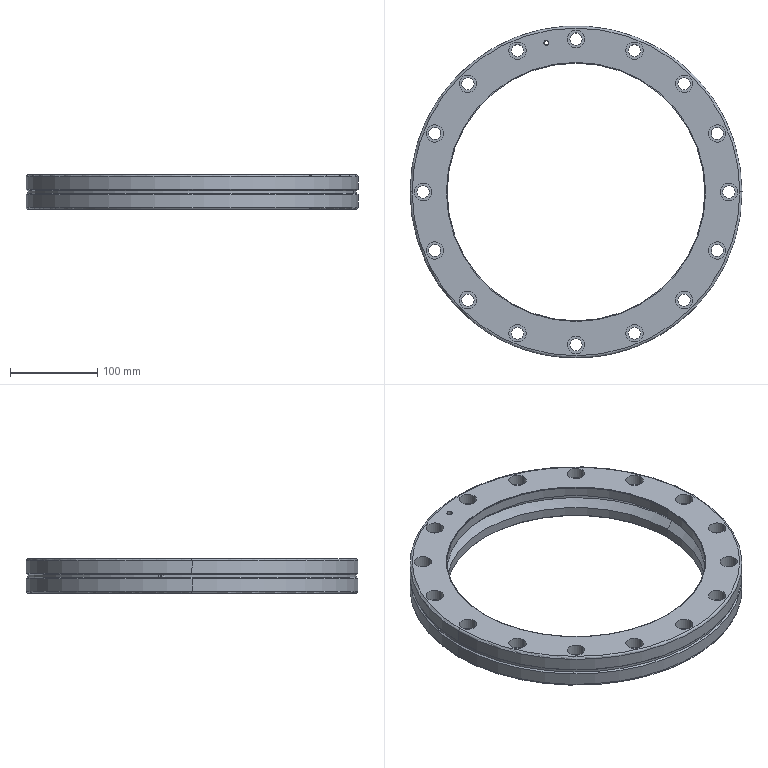Part | SolidWorks | features ICE 4, CirPattern 2, Extrusion 1, Fillet 1, HoleWzd 1, MirrorPattern 1, RefAxis 1, RevCut 1 | 1 solid | 127 faces | box 380 x 380 x 40 mm | volume 1589572 mm3 | cylinder 87 | plane 24 | cone 10 | torus 6 | commonest cylinder face diameters 14 x32 20 x32 1 x4 4 x4 295 x4 296.6 x4